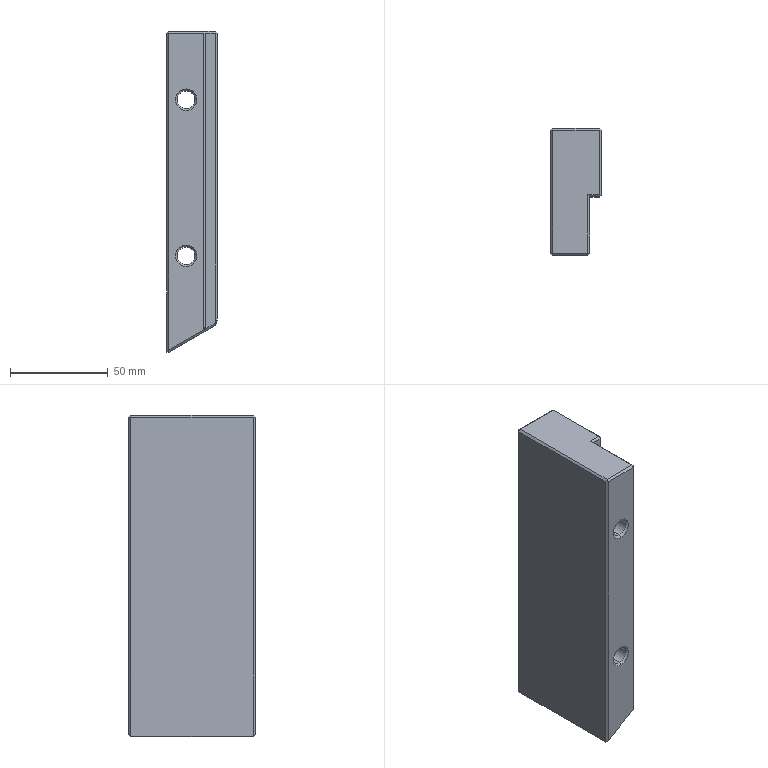Part | STEP file | Trilho - Torre - 1 cav - 2 | 1 solid | 53 faces | box 26 x 65 x 164.624 mm | volume 224436 mm3 | plane 37 | cone 8 | cylinder 8 | commonest cylinder face diameters 9 x4 15 x4